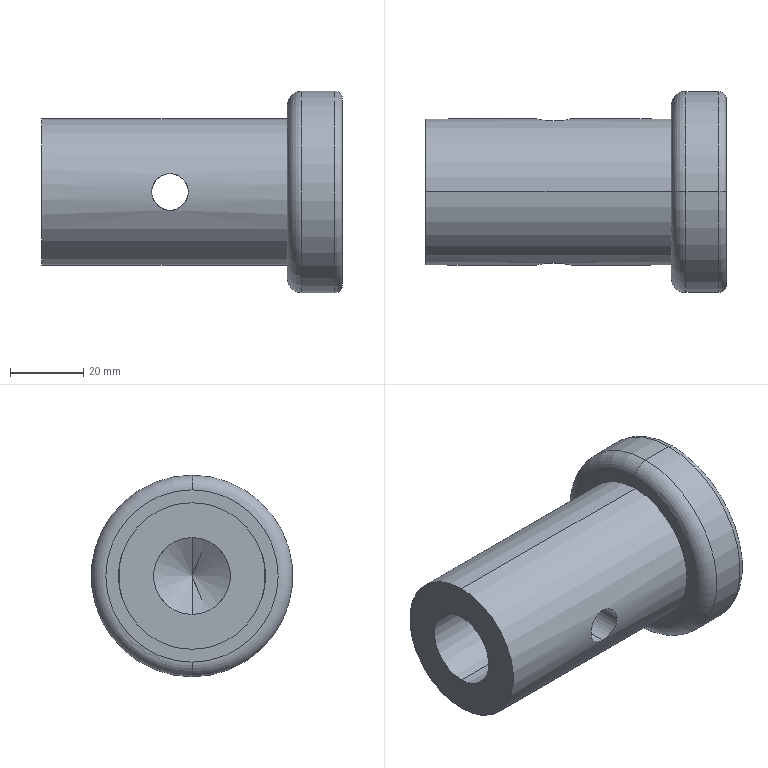Part | SolidWorks | features Fillet 2, HoleWzd 1, ICE 1, Revolution 1 | 1 solid | 21 faces | box 82 x 55 x 55 mm | volume 93090 mm3 | cylinder 10 | torus 4 | plane 3 | cone 2 | sphere 2 | commonest cylinder face diameters 10 x4 21 x2 40 x2 55 x2
STEP:
#1=CARTESIAN_POINT('',(67.,0.,23.5));
#2=VERTEX_POINT('',#1);
#3=CARTESIAN_POINT('',(67.,0.,-23.5));
#4=VERTEX_POINT('',#3);
#5=CARTESIAN_POINT('',(67.,0.,0.));
#6=DIRECTION('',(-1.,0.,0.));
#7=DIRECTION('',(0.,0.,-1.));
#8=AXIS2_PLACEMENT_3D('',#5,#6,#7);
#9=CIRCLE('',#8,23.5);
#10=EDGE_CURVE('',#2,#4,#9,.T.);
#11=ORIENTED_EDGE('',*,*,#10,.F.);
#12=CARTESIAN_POINT('',(71.,0.,27.5));
#13=VERTEX_POINT('',#12);
#14=CARTESIAN_POINT('',(71.,0.,23.5));
#15=DIRECTION('',(0.,1.,0.));
#16=DIRECTION('',(0.,0.,1.));
#17=AXIS2_PLACEMENT_3D('',#14,#15,#16);
#18=CIRCLE('',#17,4.);
#19=EDGE_CURVE('',#2,#13,#18,.T.);
#20=ORIENTED_EDGE('',*,*,#19,.T.);
#21=CARTESIAN_POINT('',(71.,0.,-27.5));
#22=VERTEX_POINT('',#21);
#23=CARTESIAN_POINT('',(71.,0.,0.));
#24=DIRECTION('',(1.,0.,0.));
#25=DIRECTION('',(0.,0.,-1.));
#26=AXIS2_PLACEMENT_3D('',#23,#24,#25);
#27=CIRCLE('',#26,27.5);
#28=EDGE_CURVE('',#22,#13,#27,.T.);
#29=ORIENTED_EDGE('',*,*,#28,.F.);
#30=CARTESIAN_POINT('',(71.,0.,-23.5));
#31=DIRECTION('',(0.,-1.,0.));
#32=DIRECTION('',(0.,0.,-1.));
#33=AXIS2_PLACEMENT_3D('',#30,#31,#32);
#34=CIRCLE('',#33,4.);
#35=EDGE_CURVE('',#4,#22,#34,.T.);
#36=ORIENTED_EDGE('',*,*,#35,.F.);
#37=EDGE_LOOP('',(#11,#20,#29,#36));
#38=FACE_OUTER_BOUND('',#37,.T.);
#39=CARTESIAN_POINT('',(71.,0.,0.));
#40=DIRECTION('',(1.,0.,0.));
#41=DIRECTION('',(0.,0.,-1.));
#42=AXIS2_PLACEMENT_3D('',#39,#40,#41);
#43=TOROIDAL_SURFACE('',#42,23.5,4.);
#44=ADVANCED_FACE('',(#38),#43,.T.);
#45=CARTESIAN_POINT('',(82.,0.,-25.5));
#46=VERTEX_POINT('',#45);
#47=CARTESIAN_POINT('',(82.,0.,25.5));
#48=VERTEX_POINT('',#47);
#49=CARTESIAN_POINT('',(82.,0.,0.));
#50=DIRECTION('',(1.,0.,0.));
#51=DIRECTION('',(0.,0.,1.));
#52=AXIS2_PLACEMENT_3D('',#49,#50,#51);
#53=CIRCLE('',#52,25.5);
#54=EDGE_CURVE('',#46,#48,#53,.T.);
#55=ORIENTED_EDGE('',*,*,#54,.F.);
#56=CARTESIAN_POINT('',(80.,0.,-27.5));
#57=VERTEX_POINT('',#56);
#58=CARTESIAN_POINT('',(80.,0.,-25.5));
#59=DIRECTION('',(0.,1.,0.));
#60=DIRECTION('',(0.,0.,1.));
#61=AXIS2_PLACEMENT_3D('',#58,#59,#60);
#62=CIRCLE('',#61,2.);
#63=EDGE_CURVE('',#46,#57,#62,.T.);
#64=ORIENTED_EDGE('',*,*,#63,.T.);
#65=CARTESIAN_POINT('',(80.,0.,27.5));
#66=VERTEX_POINT('',#65);
#67=CARTESIAN_POINT('',(80.,0.,0.));
#68=DIRECTION('',(-1.,0.,0.));
#69=DIRECTION('',(0.,0.,1.));
#70=AXIS2_PLACEMENT_3D('',#67,#68,#69);
#71=CIRCLE('',#70,27.5);
#72=EDGE_CURVE('',#66,#57,#71,.T.);
#73=ORIENTED_EDGE('',*,*,#72,.F.);
#74=CARTESIAN_POINT('',(80.,0.,25.5));
#75=DIRECTION('',(0.,-1.,0.));
#76=DIRECTION('',(0.,0.,-1.));
#77=AXIS2_PLACEMENT_3D('',#74,#75,#76);
#78=CIRCLE('',#77,2.);
#79=EDGE_CURVE('',#48,#66,#78,.T.);
#80=ORIENTED_EDGE('',*,*,#79,.F.);
#81=EDGE_LOOP('',(#55,#64,#73,#80));
#82=FACE_OUTER_BOUND('',#81,.T.);
#83=CARTESIAN_POINT('',(80.,0.,0.));
#84=DIRECTION('',(-1.,0.,0.));
#85=DIRECTION('',(0.,0.,1.));
#86=AXIS2_PLACEMENT_3D('',#83,#84,#85);
#87=TOROIDAL_SURFACE('',#86,25.5,2.);
#88=ADVANCED_FACE('',(#82),#87,.T.);
#89=CARTESIAN_POINT('',(35.,-19.365,-5.));
#90=VERTEX_POINT('',#89);
#91=CARTESIAN_POINT('',(35.,-19.365,5.));
#92=VERTEX_POINT('',#91);
#93=CARTESIAN_POINT('',(35.,-19.365,-5.));
#94=CARTESIAN_POINT('',(34.673,-19.365,-5.));
#95=CARTESIAN_POINT('',(34.347,-19.373,-4.968));
#96=CARTESIAN_POINT('',(33.697,-19.406,-4.839));
#97=CARTESIAN_POINT('',(33.385,-19.43,-4.743));
#98=CARTESIAN_POINT('',(32.782,-19.489,-4.493));
#99=CARTESIAN_POINT('',(32.49,-19.525,-4.337));
#100=CARTESIAN_POINT('',(31.948,-19.602,-3.974));
#101=CARTESIAN_POINT('',(31.697,-19.643,-3.768));
#102=CARTESIAN_POINT('',(31.236,-19.726,-3.307));
#103=CARTESIAN_POINT('',(31.025,-19.768,-3.051));
#104=CARTESIAN_POINT('',(30.664,-19.844,-2.511));
#105=CARTESIAN_POINT('',(30.51,-19.878,-2.224));
#106=CARTESIAN_POINT('',(30.257,-19.937,-1.616));
#107=CARTESIAN_POINT('',(30.161,-19.96,-1.301));
#108=CARTESIAN_POINT('',(30.065,-19.984,-0.8214));
#109=CARTESIAN_POINT('',(30.041,-19.99,-0.6596));
#110=CARTESIAN_POINT('',(30.008,-19.998,-0.3326));
#111=CARTESIAN_POINT('',(30.,-20.,-0.1664));
#112=CARTESIAN_POINT('',(30.,-20.,0.3283));
#113=CARTESIAN_POINT('',(30.032,-19.992,0.6537));
#114=CARTESIAN_POINT('',(30.16,-19.961,1.296));
#115=CARTESIAN_POINT('',(30.257,-19.937,1.615));
#116=CARTESIAN_POINT('',(30.507,-19.879,2.218));
#117=CARTESIAN_POINT('',(30.661,-19.844,2.505));
#118=CARTESIAN_POINT('',(31.025,-19.768,3.051));
#119=CARTESIAN_POINT('',(31.233,-19.727,3.304));
#120=CARTESIAN_POINT('',(31.692,-19.644,3.763));
#121=CARTESIAN_POINT('',(31.946,-19.602,3.972));
#122=CARTESIAN_POINT('',(32.49,-19.525,4.337));
#123=CARTESIAN_POINT('',(32.777,-19.49,4.49));
#124=CARTESIAN_POINT('',(33.379,-19.43,4.741));
#125=CARTESIAN_POINT('',(33.697,-19.406,4.838));
#126=CARTESIAN_POINT('',(34.341,-19.373,4.967));
#127=CARTESIAN_POINT('',(34.668,-19.365,5.));
#128=CARTESIAN_POINT('',(35.,-19.365,5.));
#129=B_SPLINE_CURVE_WITH_KNOTS('',3,(#93,#94,#95,#96,#97,#98,#99,#100,#101,#102,#103,#104,#105,#106,#107,#108,#109,#110,#111,#112,#113,#114,#115,#116,#117,#118,#119,#120,#121,#122,#123,#124,#125,#126,#127,#128),.UNSPECIFIED.,.F.,.F.,(4,2,2,2,2,2,2,2,2,2,2,2,2,2,2,2,2,4),(0.01569,0.01668,0.01766,0.01864,0.01962,0.0206,0.02158,0.02256,0.02305,0.02354,0.02452,0.0255,0.02648,0.02746,0.02844,0.02942,0.0304,0.03138),.UNSPECIFIED.);
#130=EDGE_CURVE('',#90,#92,#129,.T.);
#131=ORIENTED_EDGE('',*,*,#130,.F.);
#132=CARTESIAN_POINT('',(35.,-9.233,-5.));
#133=VERTEX_POINT('',#132);
#134=CARTESIAN_POINT('',(35.,-25.,-5.));
#135=DIRECTION('',(0.,1.,0.));
#136=VECTOR('',#135,1000.);
#137=LINE('',#134,#136);
#138=EDGE_CURVE('',#90,#133,#137,.T.);
#139=ORIENTED_EDGE('',*,*,#138,.T.);
#140=CARTESIAN_POINT('',(35.,-9.233,5.));
#141=VERTEX_POINT('',#140);
#142=CARTESIAN_POINT('',(35.,-9.233,5.));
#143=CARTESIAN_POINT('',(34.664,-9.233,5.));
#144=CARTESIAN_POINT('',(34.335,-9.251,4.966));
#145=CARTESIAN_POINT('',(33.689,-9.32,4.836));
#146=CARTESIAN_POINT('',(33.37,-9.371,4.738));
#147=CARTESIAN_POINT('',(32.767,-9.495,4.486));
#148=CARTESIAN_POINT('',(32.482,-9.567,4.332));
#149=CARTESIAN_POINT('',(31.943,-9.723,3.97));
#150=CARTESIAN_POINT('',(31.692,-9.805,3.763));
#151=CARTESIAN_POINT('',(31.238,-9.968,3.309));
#152=CARTESIAN_POINT('',(31.031,-10.049,3.059));
#153=CARTESIAN_POINT('',(30.668,-10.197,2.518));
#154=CARTESIAN_POINT('',(30.515,-10.264,2.233));
#155=CARTESIAN_POINT('',(30.326,-10.349,1.783));
#156=CARTESIAN_POINT('',(30.27,-10.374,1.629));
#157=CARTESIAN_POINT('',(30.172,-10.419,1.312));
#158=CARTESIAN_POINT('',(30.131,-10.438,1.15));
#159=CARTESIAN_POINT('',(30.033,-10.484,0.6637));
#160=CARTESIAN_POINT('',(30.,-10.5,0.3355));
#161=CARTESIAN_POINT('',(30.,-10.5,-0.1631));
#162=CARTESIAN_POINT('',(30.008,-10.496,-0.3315));
#163=CARTESIAN_POINT('',(30.041,-10.48,-0.6635));
#164=CARTESIAN_POINT('',(30.066,-10.469,-0.8273));
#165=CARTESIAN_POINT('',(30.164,-10.423,-1.312));
#166=CARTESIAN_POINT('',(30.262,-10.377,-1.63));
#167=CARTESIAN_POINT('',(30.516,-10.263,-2.237));
#168=CARTESIAN_POINT('',(30.671,-10.196,-2.523));
#169=CARTESIAN_POINT('',(31.033,-10.048,-3.061));
#170=CARTESIAN_POINT('',(31.242,-9.966,-3.314));
#171=CARTESIAN_POINT('',(31.697,-9.804,-3.768));
#172=CARTESIAN_POINT('',(31.945,-9.722,-3.972));
#173=CARTESIAN_POINT('',(32.486,-9.566,-4.334));
#174=CARTESIAN_POINT('',(32.773,-9.493,-4.488));
#175=CARTESIAN_POINT('',(33.372,-9.371,-4.739));
#176=CARTESIAN_POINT('',(33.687,-9.32,-4.836));
#177=CARTESIAN_POINT('',(34.34,-9.251,-4.967));
#178=CARTESIAN_POINT('',(34.669,-9.233,-5.));
#179=CARTESIAN_POINT('',(35.,-9.233,-5.));
#180=B_SPLINE_CURVE_WITH_KNOTS('',3,(#142,#143,#144,#145,#146,#147,#148,#149,#150,#151,#152,#153,#154,#155,#156,#157,#158,#159,#160,#161,#162,#163,#164,#165,#166,#167,#168,#169,#170,#171,#172,#173,#174,#175,#176,#177,#178,#179),.UNSPECIFIED.,.F.,.F.,(4,2,2,2,2,2,2,2,2,2,2,2,2,2,2,2,2,2,4),(0.,0.0009922,0.001984,0.002977,0.003969,0.004961,0.005953,0.006449,0.006945,0.007938,0.008434,0.00893,0.009922,0.01091,0.01191,0.0129,0.01389,0.01488,0.01588),.UNSPECIFIED.);
#181=EDGE_CURVE('',#141,#133,#180,.T.);
#182=ORIENTED_EDGE('',*,*,#181,.F.);
#183=CARTESIAN_POINT('',(35.,-25.,5.));
#184=DIRECTION('',(0.,1.,0.));
#185=VECTOR('',#184,1000.);
#186=LINE('',#183,#185);
#187=EDGE_CURVE('',#92,#141,#186,.T.);
#188=ORIENTED_EDGE('',*,*,#187,.F.);
#189=EDGE_LOOP('',(#131,#139,#182,#188));
#190=FACE_OUTER_BOUND('',#189,.T.);
#191=CARTESIAN_POINT('',(35.,-25.,0.));
#192=DIRECTION('',(0.,1.,0.));
#193=DIRECTION('',(0.,0.,1.));
#194=AXIS2_PLACEMENT_3D('',#191,#192,#193);
#195=CYLINDRICAL_SURFACE('',#194,5.);
#196=ADVANCED_FACE('',(#190),#195,.F.);
#197=CARTESIAN_POINT('',(35.,9.233,-5.));
#198=VERTEX_POINT('',#197);
#199=CARTESIAN_POINT('',(35.,9.233,5.));
#200=VERTEX_POINT('',#199);
#201=CARTESIAN_POINT('',(35.,9.233,-5.));
#202=CARTESIAN_POINT('',(34.67,9.233,-5.));
#203=CARTESIAN_POINT('',(34.333,9.252,-4.966));
#204=CARTESIAN_POINT('',(33.686,9.321,-4.835));
#205=CARTESIAN_POINT('',(33.373,9.371,-4.739));
#206=CARTESIAN_POINT('',(32.766,9.495,-4.485));
#207=CARTESIAN_POINT('',(32.48,9.568,-4.33));
#208=CARTESIAN_POINT('',(31.944,9.722,-3.971));
#209=CARTESIAN_POINT('',(31.692,9.806,-3.763));
#210=CARTESIAN_POINT('',(31.236,9.968,-3.307));
#211=CARTESIAN_POINT('',(31.032,10.048,-3.06));
#212=CARTESIAN_POINT('',(30.671,10.196,-2.523));
#213=CARTESIAN_POINT('',(30.514,10.265,-2.232));
#214=CARTESIAN_POINT('',(30.262,10.377,-1.631));
#215=CARTESIAN_POINT('',(30.166,10.422,-1.318));
#216=CARTESIAN_POINT('',(30.067,10.468,-0.8302));
#217=CARTESIAN_POINT('',(30.042,10.48,-0.664));
#218=CARTESIAN_POINT('',(30.008,10.496,-0.3336));
#219=CARTESIAN_POINT('',(29.992,10.504,-0.003189));
#220=CARTESIAN_POINT('',(30.008,10.496,0.3273));
#221=CARTESIAN_POINT('',(30.041,10.481,0.6578));
#222=CARTESIAN_POINT('',(30.066,10.469,0.824));
#223=CARTESIAN_POINT('',(30.164,10.423,1.313));
#224=CARTESIAN_POINT('',(30.261,10.378,1.626));
#225=CARTESIAN_POINT('',(30.513,10.265,2.231));
#226=CARTESIAN_POINT('',(30.671,10.196,2.522));
#227=CARTESIAN_POINT('',(31.031,10.049,3.058));
#228=CARTESIAN_POINT('',(31.237,9.968,3.308));
#229=CARTESIAN_POINT('',(31.696,9.804,3.767));
#230=CARTESIAN_POINT('',(31.944,9.722,3.971));
#231=CARTESIAN_POINT('',(32.345,9.606,4.24));
#232=CARTESIAN_POINT('',(32.483,9.569,4.324));
#233=CARTESIAN_POINT('',(32.77,9.498,4.478));
#234=CARTESIAN_POINT('',(32.919,9.464,4.549));
#235=CARTESIAN_POINT('',(33.371,9.371,4.738));
#236=CARTESIAN_POINT('',(33.682,9.321,4.834));
#237=CARTESIAN_POINT('',(34.328,9.252,4.966));
#238=CARTESIAN_POINT('',(34.665,9.233,5.));
#239=CARTESIAN_POINT('',(35.,9.233,5.));
#240=B_SPLINE_CURVE_WITH_KNOTS('',3,(#201,#202,#203,#204,#205,#206,#207,#208,#209,#210,#211,#212,#213,#214,#215,#216,#217,#218,#219,#220,#221,#222,#223,#224,#225,#226,#227,#228,#229,#230,#231,#232,#233,#234,#235,#236,#237,#238,#239),.UNSPECIFIED.,.F.,.F.,(4,2,2,2,2,2,2,2,2,1,2,2,2,2,2,2,2,2,2,4),(0.01588,0.01687,0.01786,0.01885,0.01984,0.02083,0.02182,0.02281,0.02331,0.0238,0.0243,0.02479,0.02578,0.02677,0.02776,0.02876,0.02925,0.02975,0.03074,0.03173),.UNSPECIFIED.);
#241=EDGE_CURVE('',#198,#200,#240,.T.);
#242=ORIENTED_EDGE('',*,*,#241,.F.);
#243=CARTESIAN_POINT('',(35.,19.365,-5.));
#244=VERTEX_POINT('',#243);
#245=CARTESIAN_POINT('',(35.,-25.,-5.));
#246=DIRECTION('',(0.,1.,0.));
#247=VECTOR('',#246,1000.);
#248=LINE('',#245,#247);
#249=EDGE_CURVE('',#198,#244,#248,.T.);
#250=ORIENTED_EDGE('',*,*,#249,.T.);
#251=CARTESIAN_POINT('',(35.,19.365,5.));
#252=VERTEX_POINT('',#251);
#253=CARTESIAN_POINT('',(35.,19.365,5.));
#254=CARTESIAN_POINT('',(34.668,19.365,5.));
#255=CARTESIAN_POINT('',(34.342,19.373,4.967));
#256=CARTESIAN_POINT('',(33.701,19.406,4.839));
#257=CARTESIAN_POINT('',(33.383,19.43,4.743));
#258=CARTESIAN_POINT('',(32.778,19.49,4.491));
#259=CARTESIAN_POINT('',(32.492,19.525,4.338));
#260=CARTESIAN_POINT('',(31.949,19.602,3.975));
#261=CARTESIAN_POINT('',(31.693,19.644,3.764));
#262=CARTESIAN_POINT('',(31.234,19.726,3.305));
#263=CARTESIAN_POINT('',(31.028,19.767,3.054));
#264=CARTESIAN_POINT('',(30.662,19.844,2.508));
#265=CARTESIAN_POINT('',(30.508,19.879,2.219));
#266=CARTESIAN_POINT('',(30.32,19.922,1.768));
#267=CARTESIAN_POINT('',(30.265,19.935,1.614));
#268=CARTESIAN_POINT('',(30.169,19.958,1.301));
#269=CARTESIAN_POINT('',(30.129,19.968,1.14));
#270=CARTESIAN_POINT('',(30.032,19.992,0.655));
#271=CARTESIAN_POINT('',(30.,20.,0.3296));
#272=CARTESIAN_POINT('',(30.,20.,-0.3256));
#273=CARTESIAN_POINT('',(30.033,19.992,-0.6584));
#274=CARTESIAN_POINT('',(30.161,19.96,-1.301));
#275=CARTESIAN_POINT('',(30.256,19.937,-1.613));
#276=CARTESIAN_POINT('',(30.508,19.879,-2.22));
#277=CARTESIAN_POINT('',(30.664,19.844,-2.511));
#278=CARTESIAN_POINT('',(31.025,19.768,-3.051));
#279=CARTESIAN_POINT('',(31.234,19.726,-3.305));
#280=CARTESIAN_POINT('',(31.697,19.643,-3.768));
#281=CARTESIAN_POINT('',(31.948,19.602,-3.974));
#282=CARTESIAN_POINT('',(32.489,19.525,-4.336));
#283=CARTESIAN_POINT('',(32.782,19.489,-4.493));
#284=CARTESIAN_POINT('',(33.385,19.43,-4.743));
#285=CARTESIAN_POINT('',(33.697,19.406,-4.838));
#286=CARTESIAN_POINT('',(34.18,19.382,-4.935));
#287=CARTESIAN_POINT('',(34.344,19.375,-4.96));
#288=CARTESIAN_POINT('',(34.673,19.367,-4.992));
#289=CARTESIAN_POINT('',(34.836,19.365,-5.));
#290=CARTESIAN_POINT('',(35.,19.365,-5.));
#291=B_SPLINE_CURVE_WITH_KNOTS('',3,(#253,#254,#255,#256,#257,#258,#259,#260,#261,#262,#263,#264,#265,#266,#267,#268,#269,#270,#271,#272,#273,#274,#275,#276,#277,#278,#279,#280,#281,#282,#283,#284,#285,#286,#287,#288,#289,#290),.UNSPECIFIED.,.F.,.F.,(4,2,2,2,2,2,2,2,2,2,2,2,2,2,2,2,2,2,4),(0.,0.0009809,0.001962,0.002943,0.003924,0.004905,0.005885,0.006376,0.006866,0.007847,0.008828,0.009809,0.01079,0.01177,0.01275,0.01373,0.01471,0.0152,0.01569),.UNSPECIFIED.);
#292=EDGE_CURVE('',#252,#244,#291,.T.);
#293=ORIENTED_EDGE('',*,*,#292,.F.);
#294=CARTESIAN_POINT('',(35.,-25.,5.));
#295=DIRECTION('',(0.,1.,0.));
#296=VECTOR('',#295,1000.);
#297=LINE('',#294,#296);
#298=EDGE_CURVE('',#200,#252,#297,.T.);
#299=ORIENTED_EDGE('',*,*,#298,.F.);
#300=EDGE_LOOP('',(#242,#250,#293,#299));
#301=FACE_OUTER_BOUND('',#300,.T.);
#302=CARTESIAN_POINT('',(35.,-25.,0.));
#303=DIRECTION('',(0.,1.,0.));
#304=DIRECTION('',(0.,0.,1.));
#305=AXIS2_PLACEMENT_3D('',#302,#303,#304);
#306=CYLINDRICAL_SURFACE('',#305,5.);
#307=ADVANCED_FACE('',(#301),#306,.F.);
#308=ORIENTED_EDGE('',*,*,#181,.T.);
#309=CARTESIAN_POINT('',(35.,-9.233,-5.));
#310=CARTESIAN_POINT('',(35.33,-9.233,-5.));
#311=CARTESIAN_POINT('',(35.667,-9.252,-4.966));
#312=CARTESIAN_POINT('',(36.314,-9.321,-4.835));
#313=CARTESIAN_POINT('',(36.627,-9.371,-4.739));
#314=CARTESIAN_POINT('',(37.234,-9.495,-4.485));
#315=CARTESIAN_POINT('',(37.52,-9.568,-4.33));
#316=CARTESIAN_POINT('',(38.056,-9.722,-3.971));
#317=CARTESIAN_POINT('',(38.308,-9.806,-3.763));
#318=CARTESIAN_POINT('',(38.764,-9.968,-3.307));
#319=CARTESIAN_POINT('',(38.968,-10.048,-3.06));
#320=CARTESIAN_POINT('',(39.329,-10.196,-2.523));
#321=CARTESIAN_POINT('',(39.486,-10.265,-2.232));
#322=CARTESIAN_POINT('',(39.738,-10.377,-1.631));
#323=CARTESIAN_POINT('',(39.834,-10.422,-1.318));
#324=CARTESIAN_POINT('',(39.933,-10.468,-0.8302));
#325=CARTESIAN_POINT('',(39.958,-10.48,-0.664));
#326=CARTESIAN_POINT('',(39.992,-10.496,-0.3336));
#327=CARTESIAN_POINT('',(40.008,-10.504,-0.003189));
#328=CARTESIAN_POINT('',(39.992,-10.496,0.3273));
#329=CARTESIAN_POINT('',(39.959,-10.481,0.6578));
#330=CARTESIAN_POINT('',(39.934,-10.469,0.824));
#331=CARTESIAN_POINT('',(39.836,-10.423,1.313));
#332=CARTESIAN_POINT('',(39.739,-10.378,1.626));
#333=CARTESIAN_POINT('',(39.487,-10.265,2.231));
#334=CARTESIAN_POINT('',(39.329,-10.196,2.522));
#335=CARTESIAN_POINT('',(38.969,-10.049,3.058));
#336=CARTESIAN_POINT('',(38.763,-9.968,3.308));
#337=CARTESIAN_POINT('',(38.304,-9.804,3.767));
#338=CARTESIAN_POINT('',(38.056,-9.722,3.971));
#339=CARTESIAN_POINT('',(37.655,-9.606,4.24));
#340=CARTESIAN_POINT('',(37.517,-9.569,4.324));
#341=CARTESIAN_POINT('',(37.23,-9.498,4.478));
#342=CARTESIAN_POINT('',(37.081,-9.464,4.549));
#343=CARTESIAN_POINT('',(36.629,-9.371,4.738));
#344=CARTESIAN_POINT('',(36.318,-9.321,4.834));
#345=CARTESIAN_POINT('',(35.672,-9.252,4.966));
#346=CARTESIAN_POINT('',(35.335,-9.233,5.));
#347=CARTESIAN_POINT('',(35.,-9.233,5.));
#348=B_SPLINE_CURVE_WITH_KNOTS('',3,(#309,#310,#311,#312,#313,#314,#315,#316,#317,#318,#319,#320,#321,#322,#323,#324,#325,#326,#327,#328,#329,#330,#331,#332,#333,#334,#335,#336,#337,#338,#339,#340,#341,#342,#343,#344,#345,#346,#347),.UNSPECIFIED.,.F.,.F.,(4,2,2,2,2,2,2,2,2,1,2,2,2,2,2,2,2,2,2,4),(0.01588,0.01687,0.01786,0.01885,0.01984,0.02083,0.02182,0.02281,0.02331,0.0238,0.0243,0.02479,0.02578,0.02677,0.02776,0.02876,0.02925,0.02975,0.03074,0.03173),.UNSPECIFIED.);
#349=EDGE_CURVE('',#133,#141,#348,.T.);
#350=ORIENTED_EDGE('',*,*,#349,.T.);
#351=EDGE_LOOP('',(#308,#350));
#352=FACE_BOUND('',#351,.T.);
#353=CARTESIAN_POINT('',(57.,0.,-10.5));
#354=VERTEX_POINT('',#353);
#355=CARTESIAN_POINT('',(57.,0.,10.5));
#356=VERTEX_POINT('',#355);
#357=CARTESIAN_POINT('',(57.,0.,0.));
#358=DIRECTION('',(-1.,0.,0.));
#359=DIRECTION('',(0.,0.,1.));
#360=AXIS2_PLACEMENT_3D('',#357,#358,#359);
#361=CIRCLE('',#360,10.5);
#362=EDGE_CURVE('',#354,#356,#361,.T.);
#363=ORIENTED_EDGE('',*,*,#362,.F.);
#364=CARTESIAN_POINT('',(0.,0.,-10.5));
#365=VERTEX_POINT('',#364);
#366=CARTESIAN_POINT('',(0.,0.,-10.5));
#367=DIRECTION('',(-1.,0.,0.));
#368=VECTOR('',#367,1000.);
#369=LINE('',#366,#368);
#370=EDGE_CURVE('',#354,#365,#369,.T.);
#371=ORIENTED_EDGE('',*,*,#370,.T.);
#372=CARTESIAN_POINT('',(0.,0.,10.5));
#373=VERTEX_POINT('',#372);
#374=CARTESIAN_POINT('',(0.,0.,0.));
#375=DIRECTION('',(-1.,0.,0.));
#376=DIRECTION('',(0.,0.,1.));
#377=AXIS2_PLACEMENT_3D('',#374,#375,#376);
#378=CIRCLE('',#377,10.5);
#379=EDGE_CURVE('',#365,#373,#378,.T.);
#380=ORIENTED_EDGE('',*,*,#379,.T.);
#381=CARTESIAN_POINT('',(0.,0.,10.5));
#382=DIRECTION('',(-1.,0.,0.));
#383=VECTOR('',#382,1000.);
#384=LINE('',#381,#383);
#385=EDGE_CURVE('',#356,#373,#384,.T.);
#386=ORIENTED_EDGE('',*,*,#385,.F.);
#387=EDGE_LOOP('',(#363,#371,#380,#386));
#388=FACE_OUTER_BOUND('',#387,.T.);
#389=CARTESIAN_POINT('',(0.,0.,0.));
#390=DIRECTION('',(-1.,0.,0.));
#391=DIRECTION('',(0.,0.,1.));
#392=AXIS2_PLACEMENT_3D('',#389,#390,#391);
#393=CYLINDRICAL_SURFACE('',#392,10.5);
#394=ADVANCED_FACE('',(#352,#388),#393,.F.);
#395=CARTESIAN_POINT('',(63.309,0.,0.));
#396=VERTEX_POINT('',#395);
#397=CARTESIAN_POINT('',(57.,0.,10.5));
#398=DIRECTION('',(-0.515,0.,0.8572));
#399=VECTOR('',#398,1000.);
#400=LINE('',#397,#399);
#401=EDGE_CURVE('',#396,#356,#400,.T.);
#402=ORIENTED_EDGE('',*,*,#401,.F.);
#403=CARTESIAN_POINT('',(57.,0.,-10.5));
#404=DIRECTION('',(-0.515,0.,-0.8572));
#405=VECTOR('',#404,1000.);
#406=LINE('',#403,#405);
#407=EDGE_CURVE('',#396,#354,#406,.T.);
#408=ORIENTED_EDGE('',*,*,#407,.T.);
#409=ORIENTED_EDGE('',*,*,#362,.T.);
#410=EDGE_LOOP('',(#402,#408,#409));
#411=FACE_OUTER_BOUND('',#410,.T.);
#412=CARTESIAN_POINT('',(57.,0.,0.));
#413=DIRECTION('',(-1.,0.,0.));
#414=DIRECTION('',(0.,0.,1.));
#415=AXIS2_PLACEMENT_3D('',#412,#413,#414);
#416=CONICAL_SURFACE('',#415,10.5,1.03);
#417=ADVANCED_FACE('',(#411),#416,.F.);
#418=ORIENTED_EDGE('',*,*,#292,.T.);
#419=CARTESIAN_POINT('',(35.,19.365,-5.));
#420=CARTESIAN_POINT('',(35.327,19.365,-5.));
#421=CARTESIAN_POINT('',(35.653,19.373,-4.968));
#422=CARTESIAN_POINT('',(36.303,19.406,-4.839));
#423=CARTESIAN_POINT('',(36.615,19.43,-4.743));
#424=CARTESIAN_POINT('',(37.218,19.489,-4.493));
#425=CARTESIAN_POINT('',(37.51,19.525,-4.337));
#426=CARTESIAN_POINT('',(38.052,19.602,-3.974));
#427=CARTESIAN_POINT('',(38.303,19.643,-3.768));
#428=CARTESIAN_POINT('',(38.764,19.726,-3.307));
#429=CARTESIAN_POINT('',(38.975,19.768,-3.051));
#430=CARTESIAN_POINT('',(39.336,19.844,-2.511));
#431=CARTESIAN_POINT('',(39.49,19.878,-2.224));
#432=CARTESIAN_POINT('',(39.743,19.937,-1.616));
#433=CARTESIAN_POINT('',(39.839,19.96,-1.301));
#434=CARTESIAN_POINT('',(39.935,19.984,-0.8214));
#435=CARTESIAN_POINT('',(39.959,19.99,-0.6596));
#436=CARTESIAN_POINT('',(39.992,19.998,-0.3326));
#437=CARTESIAN_POINT('',(40.,20.,-0.1664));
#438=CARTESIAN_POINT('',(40.,20.,0.3283));
#439=CARTESIAN_POINT('',(39.968,19.992,0.6537));
#440=CARTESIAN_POINT('',(39.84,19.961,1.296));
#441=CARTESIAN_POINT('',(39.743,19.937,1.615));
#442=CARTESIAN_POINT('',(39.493,19.879,2.218));
#443=CARTESIAN_POINT('',(39.339,19.844,2.505));
#444=CARTESIAN_POINT('',(38.975,19.768,3.051));
#445=CARTESIAN_POINT('',(38.767,19.727,3.304));
#446=CARTESIAN_POINT('',(38.308,19.644,3.763));
#447=CARTESIAN_POINT('',(38.054,19.602,3.972));
#448=CARTESIAN_POINT('',(37.51,19.525,4.337));
#449=CARTESIAN_POINT('',(37.223,19.49,4.49));
#450=CARTESIAN_POINT('',(36.621,19.43,4.741));
#451=CARTESIAN_POINT('',(36.303,19.406,4.838));
#452=CARTESIAN_POINT('',(35.659,19.373,4.967));
#453=CARTESIAN_POINT('',(35.332,19.365,5.));
#454=CARTESIAN_POINT('',(35.,19.365,5.));
#455=B_SPLINE_CURVE_WITH_KNOTS('',3,(#419,#420,#421,#422,#423,#424,#425,#426,#427,#428,#429,#430,#431,#432,#433,#434,#435,#436,#437,#438,#439,#440,#441,#442,#443,#444,#445,#446,#447,#448,#449,#450,#451,#452,#453,#454),.UNSPECIFIED.,.F.,.F.,(4,2,2,2,2,2,2,2,2,2,2,2,2,2,2,2,2,4),(0.01569,0.01668,0.01766,0.01864,0.01962,0.0206,0.02158,0.02256,0.02305,0.02354,0.02452,0.0255,0.02648,0.02746,0.02844,0.02942,0.0304,0.03138),.UNSPECIFIED.);
#456=EDGE_CURVE('',#244,#252,#455,.T.);
#457=ORIENTED_EDGE('',*,*,#456,.T.);
#458=EDGE_LOOP('',(#418,#457));
#459=FACE_BOUND('',#458,.T.);
#460=CARTESIAN_POINT('',(67.,0.,20.));
#461=VERTEX_POINT('',#460);
#462=CARTESIAN_POINT('',(67.,0.,-20.));
#463=VERTEX_POINT('',#462);
#464=CARTESIAN_POINT('',(67.,0.,0.));
#465=DIRECTION('',(-1.,0.,0.));
#466=DIRECTION('',(0.,0.,1.));
#467=AXIS2_PLACEMENT_3D('',#464,#465,#466);
#468=CIRCLE('',#467,20.);
#469=EDGE_CURVE('',#461,#463,#468,.T.);
#470=ORIENTED_EDGE('',*,*,#469,.T.);
#471=CARTESIAN_POINT('',(0.,0.,-20.));
#472=VERTEX_POINT('',#471);
#473=CARTESIAN_POINT('',(0.,0.,-20.));
#474=DIRECTION('',(-1.,0.,0.));
#475=VECTOR('',#474,1000.);
#476=LINE('',#473,#475);
#477=EDGE_CURVE('',#463,#472,#476,.T.);
#478=ORIENTED_EDGE('',*,*,#477,.T.);
#479=CARTESIAN_POINT('',(0.,0.,20.));
#480=VERTEX_POINT('',#479);
#481=CARTESIAN_POINT('',(0.,0.,0.));
#482=DIRECTION('',(-1.,0.,0.));
#483=DIRECTION('',(0.,0.,1.));
#484=AXIS2_PLACEMENT_3D('',#481,#482,#483);
#485=CIRCLE('',#484,20.);
#486=EDGE_CURVE('',#480,#472,#485,.T.);
#487=ORIENTED_EDGE('',*,*,#486,.F.);
#488=CARTESIAN_POINT('',(0.,0.,20.));
#489=DIRECTION('',(-1.,0.,0.));
#490=VECTOR('',#489,1000.);
#491=LINE('',#488,#490);
#492=EDGE_CURVE('',#461,#480,#491,.T.);
#493=ORIENTED_EDGE('',*,*,#492,.F.);
#494=EDGE_LOOP('',(#470,#478,#487,#493));
#495=FACE_OUTER_BOUND('',#494,.T.);
#496=CARTESIAN_POINT('',(0.,0.,0.));
#497=DIRECTION('',(-1.,0.,0.));
#498=DIRECTION('',(0.,0.,1.));
#499=AXIS2_PLACEMENT_3D('',#496,#497,#498);
#500=CYLINDRICAL_SURFACE('',#499,20.);
#501=ADVANCED_FACE('',(#459,#495),#500,.T.);
#502=ORIENTED_EDGE('',*,*,#72,.T.);
#503=CARTESIAN_POINT('',(0.,0.,-27.5));
#504=DIRECTION('',(-1.,0.,0.));
#505=VECTOR('',#504,1000.);
#506=LINE('',#503,#505);
#507=EDGE_CURVE('',#57,#22,#506,.T.);
#508=ORIENTED_EDGE('',*,*,#507,.T.);
#509=ORIENTED_EDGE('',*,*,#28,.T.);
#510=CARTESIAN_POINT('',(0.,0.,27.5));
#511=DIRECTION('',(-1.,0.,0.));
#512=VECTOR('',#511,1000.);
#513=LINE('',#510,#512);
#514=EDGE_CURVE('',#66,#13,#513,.T.);
#515=ORIENTED_EDGE('',*,*,#514,.F.);
#516=EDGE_LOOP('',(#502,#508,#509,#515));
#517=FACE_OUTER_BOUND('',#516,.T.);
#518=CARTESIAN_POINT('',(0.,0.,0.));
#519=DIRECTION('',(-1.,0.,0.));
#520=DIRECTION('',(0.,0.,1.));
#521=AXIS2_PLACEMENT_3D('',#518,#519,#520);
#522=CYLINDRICAL_SURFACE('',#521,27.5);
#523=ADVANCED_FACE('',(#517),#522,.T.);
#524=CARTESIAN_POINT('',(82.,24.,0.));
#525=VERTEX_POINT('',#524);
#526=CARTESIAN_POINT('',(82.,-24.,0.));
#527=VERTEX_POINT('',#526);
#528=CARTESIAN_POINT('',(82.,0.,0.));
#529=DIRECTION('',(-1.,0.,0.));
#530=DIRECTION('',(0.,0.,1.));
#531=AXIS2_PLACEMENT_3D('',#528,#529,#530);
#532=CIRCLE('',#531,24.);
#533=EDGE_CURVE('',#525,#527,#532,.T.);
#534=ORIENTED_EDGE('',*,*,#533,.F.);
#535=CARTESIAN_POINT('',(77.589,0.,0.));
#536=VERTEX_POINT('',#535);
#537=CARTESIAN_POINT('',(145.089,0.,0.));
#538=DIRECTION('',(0.,0.,1.));
#539=DIRECTION('',(0.,-1.,0.));
#540=AXIS2_PLACEMENT_3D('',#537,#538,#539);
#541=CIRCLE('',#540,67.5);
#542=EDGE_CURVE('',#525,#536,#541,.T.);
#543=ORIENTED_EDGE('',*,*,#542,.T.);
#544=CARTESIAN_POINT('',(145.089,0.,0.));
#545=DIRECTION('',(0.,0.,-1.));
#546=DIRECTION('',(-1.,0.,0.));
#547=AXIS2_PLACEMENT_3D('',#544,#545,#546);
#548=CIRCLE('',#547,67.5);
#549=EDGE_CURVE('',#527,#536,#548,.T.);
#550=ORIENTED_EDGE('',*,*,#549,.F.);
#551=EDGE_LOOP('',(#534,#543,#550));
#552=FACE_OUTER_BOUND('',#551,.T.);
#553=CARTESIAN_POINT('',(145.089,0.,0.));
#554=DIRECTION('',(0.,0.,1.));
#555=DIRECTION('',(0.,-1.,0.));
#556=AXIS2_PLACEMENT_3D('',#553,#554,#555);
#557=SPHERICAL_SURFACE('',#556,67.5);
#558=ADVANCED_FACE('',(#552),#557,.F.);
#559=CARTESIAN_POINT('',(0.,0.,0.));
#560=DIRECTION('',(-1.,0.,0.));
#561=DIRECTION('',(0.,0.,1.));
#562=AXIS2_PLACEMENT_3D('',#559,#560,#561);
#563=CIRCLE('',#562,10.5);
#564=EDGE_CURVE('',#373,#365,#563,.T.);
#565=ORIENTED_EDGE('',*,*,#564,.F.);
#566=ORIENTED_EDGE('',*,*,#379,.F.);
#567=EDGE_LOOP('',(#565,#566));
#568=FACE_BOUND('',#567,.T.);
#569=ORIENTED_EDGE('',*,*,#486,.T.);
#570=CARTESIAN_POINT('',(0.,0.,0.));
#571=DIRECTION('',(-1.,0.,0.));
#572=DIRECTION('',(0.,0.,1.));
#573=AXIS2_PLACEMENT_3D('',#570,#571,#572);
#574=CIRCLE('',#573,20.);
#575=EDGE_CURVE('',#472,#480,#574,.T.);
#576=ORIENTED_EDGE('',*,*,#575,.T.);
#577=EDGE_LOOP('',(#569,#576));
#578=FACE_OUTER_BOUND('',#577,.T.);
#579=CARTESIAN_POINT('',(0.,0.,0.));
#580=DIRECTION('',(1.,0.,0.));
#581=DIRECTION('',(0.,0.,-1.));
#582=AXIS2_PLACEMENT_3D('',#579,#580,#581);
#583=PLANE('',#582);
#584=ADVANCED_FACE('',(#568,#578),#583,.F.);
#585=ORIENTED_EDGE('',*,*,#542,.F.);
#586=CARTESIAN_POINT('',(82.,0.,0.));
#587=DIRECTION('',(-1.,0.,0.));
#588=DIRECTION('',(0.,0.,1.));
#589=AXIS2_PLACEMENT_3D('',#586,#587,#588);
#590=CIRCLE('',#589,24.);
#591=EDGE_CURVE('',#527,#525,#590,.T.);
#592=ORIENTED_EDGE('',*,*,#591,.F.);
#593=ORIENTED_EDGE('',*,*,#549,.T.);
#594=EDGE_LOOP('',(#585,#592,#593));
#595=FACE_OUTER_BOUND('',#594,.T.);
#596=CARTESIAN_POINT('',(145.089,0.,0.));
#597=DIRECTION('',(0.,0.,1.));
#598=DIRECTION('',(0.,-1.,0.));
#599=AXIS2_PLACEMENT_3D('',#596,#597,#598);
#600=SPHERICAL_SURFACE('',#599,67.5);
#601=ADVANCED_FACE('',(#595),#600,.F.);
#602=CARTESIAN_POINT('',(82.,0.,0.));
#603=DIRECTION('',(1.,0.,0.));
#604=DIRECTION('',(0.,0.,1.));
#605=AXIS2_PLACEMENT_3D('',#602,#603,#604);
#606=CIRCLE('',#605,25.5);
#607=EDGE_CURVE('',#48,#46,#606,.T.);
#608=ORIENTED_EDGE('',*,*,#607,.T.);
#609=ORIENTED_EDGE('',*,*,#54,.T.);
#610=EDGE_LOOP('',(#608,#609));
#611=FACE_OUTER_BOUND('',#610,.T.);
#612=ORIENTED_EDGE('',*,*,#591,.T.);
#613=ORIENTED_EDGE('',*,*,#533,.T.);
#614=EDGE_LOOP('',(#612,#613));
#615=FACE_BOUND('',#614,.T.);
#616=CARTESIAN_POINT('',(82.,24.,0.));
#617=DIRECTION('',(-1.,0.,0.));
#618=DIRECTION('',(0.,0.,1.));
#619=AXIS2_PLACEMENT_3D('',#616,#617,#618);
#620=PLANE('',#619);
#621=ADVANCED_FACE('',(#611,#615),#620,.F.);
#622=ORIENTED_EDGE('',*,*,#507,.F.);
#623=CARTESIAN_POINT('',(80.,0.,0.));
#624=DIRECTION('',(-1.,0.,0.));
#625=DIRECTION('',(0.,0.,1.));
#626=AXIS2_PLACEMENT_3D('',#623,#624,#625);
#627=CIRCLE('',#626,27.5);
#628=EDGE_CURVE('',#57,#66,#627,.T.);
#629=ORIENTED_EDGE('',*,*,#628,.T.);
#630=ORIENTED_EDGE('',*,*,#514,.T.);
#631=CARTESIAN_POINT('',(71.,0.,0.));
#632=DIRECTION('',(1.,0.,0.));
#633=DIRECTION('',(0.,0.,-1.));
#634=AXIS2_PLACEMENT_3D('',#631,#632,#633);
#635=CIRCLE('',#634,27.5);
#636=EDGE_CURVE('',#13,#22,#635,.T.);
#637=ORIENTED_EDGE('',*,*,#636,.T.);
#638=EDGE_LOOP('',(#622,#629,#630,#637));
#639=FACE_OUTER_BOUND('',#638,.T.);
#640=CARTESIAN_POINT('',(0.,0.,0.));
#641=DIRECTION('',(-1.,0.,0.));
#642=DIRECTION('',(0.,0.,1.));
#643=AXIS2_PLACEMENT_3D('',#640,#641,#642);
#644=CYLINDRICAL_SURFACE('',#643,27.5);
#645=ADVANCED_FACE('',(#639),#644,.T.);
#646=CARTESIAN_POINT('',(67.,0.,0.));
#647=DIRECTION('',(-1.,0.,0.));
#648=DIRECTION('',(0.,0.,-1.));
#649=AXIS2_PLACEMENT_3D('',#646,#647,#648);
#650=CIRCLE('',#649,23.5);
#651=EDGE_CURVE('',#4,#2,#650,.T.);
#652=ORIENTED_EDGE('',*,*,#651,.T.);
#653=ORIENTED_EDGE('',*,*,#10,.T.);
#654=EDGE_LOOP('',(#652,#653));
#655=FACE_OUTER_BOUND('',#654,.T.);
#656=ORIENTED_EDGE('',*,*,#469,.F.);
#657=CARTESIAN_POINT('',(67.,0.,0.));
#658=DIRECTION('',(-1.,0.,0.));
#659=DIRECTION('',(0.,0.,1.));
#660=AXIS2_PLACEMENT_3D('',#657,#658,#659);
#661=CIRCLE('',#660,20.);
#662=EDGE_CURVE('',#463,#461,#661,.T.);
#663=ORIENTED_EDGE('',*,*,#662,.F.);
#664=EDGE_LOOP('',(#656,#663));
#665=FACE_BOUND('',#664,.T.);
#666=CARTESIAN_POINT('',(67.,27.5,0.));
#667=DIRECTION('',(1.,0.,0.));
#668=DIRECTION('',(0.,0.,-1.));
#669=AXIS2_PLACEMENT_3D('',#666,#667,#668);
#670=PLANE('',#669);
#671=ADVANCED_FACE('',(#655,#665),#670,.F.);
#672=ORIENTED_EDGE('',*,*,#477,.F.);
#673=ORIENTED_EDGE('',*,*,#662,.T.);
#674=ORIENTED_EDGE('',*,*,#492,.T.);
#675=ORIENTED_EDGE('',*,*,#575,.F.);
#676=EDGE_LOOP('',(#672,#673,#674,#675));
#677=FACE_OUTER_BOUND('',#676,.T.);
#678=CARTESIAN_POINT('',(35.,-19.365,5.));
#679=CARTESIAN_POINT('',(35.332,-19.365,5.));
#680=CARTESIAN_POINT('',(35.658,-19.373,4.967));
#681=CARTESIAN_POINT('',(36.299,-19.406,4.839));
#682=CARTESIAN_POINT('',(36.617,-19.43,4.743));
#683=CARTESIAN_POINT('',(37.222,-19.49,4.491));
#684=CARTESIAN_POINT('',(37.508,-19.525,4.338));
#685=CARTESIAN_POINT('',(38.051,-19.602,3.975));
#686=CARTESIAN_POINT('',(38.307,-19.644,3.764));
#687=CARTESIAN_POINT('',(38.766,-19.726,3.305));
#688=CARTESIAN_POINT('',(38.972,-19.767,3.054));
#689=CARTESIAN_POINT('',(39.338,-19.844,2.508));
#690=CARTESIAN_POINT('',(39.492,-19.879,2.219));
#691=CARTESIAN_POINT('',(39.68,-19.922,1.768));
#692=CARTESIAN_POINT('',(39.735,-19.935,1.614));
#693=CARTESIAN_POINT('',(39.831,-19.958,1.301));
#694=CARTESIAN_POINT('',(39.871,-19.968,1.14));
#695=CARTESIAN_POINT('',(39.968,-19.992,0.655));
#696=CARTESIAN_POINT('',(40.,-20.,0.3296));
#697=CARTESIAN_POINT('',(40.,-20.,-0.3256));
#698=CARTESIAN_POINT('',(39.967,-19.992,-0.6584));
#699=CARTESIAN_POINT('',(39.839,-19.96,-1.301));
#700=CARTESIAN_POINT('',(39.744,-19.937,-1.613));
#701=CARTESIAN_POINT('',(39.492,-19.879,-2.22));
#702=CARTESIAN_POINT('',(39.336,-19.844,-2.511));
#703=CARTESIAN_POINT('',(38.975,-19.768,-3.051));
#704=CARTESIAN_POINT('',(38.766,-19.726,-3.305));
#705=CARTESIAN_POINT('',(38.303,-19.643,-3.768));
#706=CARTESIAN_POINT('',(38.052,-19.602,-3.974));
#707=CARTESIAN_POINT('',(37.511,-19.525,-4.336));
#708=CARTESIAN_POINT('',(37.218,-19.489,-4.493));
#709=CARTESIAN_POINT('',(36.615,-19.43,-4.743));
#710=CARTESIAN_POINT('',(36.303,-19.406,-4.838));
#711=CARTESIAN_POINT('',(35.82,-19.382,-4.935));
#712=CARTESIAN_POINT('',(35.656,-19.375,-4.96));
#713=CARTESIAN_POINT('',(35.327,-19.367,-4.992));
#714=CARTESIAN_POINT('',(35.164,-19.365,-5.));
#715=CARTESIAN_POINT('',(35.,-19.365,-5.));
#716=B_SPLINE_CURVE_WITH_KNOTS('',3,(#678,#679,#680,#681,#682,#683,#684,#685,#686,#687,#688,#689,#690,#691,#692,#693,#694,#695,#696,#697,#698,#699,#700,#701,#702,#703,#704,#705,#706,#707,#708,#709,#710,#711,#712,#713,#714,#715),.UNSPECIFIED.,.F.,.F.,(4,2,2,2,2,2,2,2,2,2,2,2,2,2,2,2,2,2,4),(0.,0.0009809,0.001962,0.002943,0.003924,0.004905,0.005885,0.006376,0.006866,0.007847,0.008828,0.009809,0.01079,0.01177,0.01275,0.01373,0.01471,0.0152,0.01569),.UNSPECIFIED.);
#717=EDGE_CURVE('',#92,#90,#716,.T.);
#718=ORIENTED_EDGE('',*,*,#717,.T.);
#719=ORIENTED_EDGE('',*,*,#130,.T.);
#720=EDGE_LOOP('',(#718,#719));
#721=FACE_BOUND('',#720,.T.);
#722=CARTESIAN_POINT('',(0.,0.,0.));
#723=DIRECTION('',(-1.,0.,0.));
#724=DIRECTION('',(0.,0.,1.));
#725=AXIS2_PLACEMENT_3D('',#722,#723,#724);
#726=CYLINDRICAL_SURFACE('',#725,20.);
#727=ADVANCED_FACE('',(#677,#721),#726,.T.);
#728=ORIENTED_EDGE('',*,*,#407,.F.);
#729=ORIENTED_EDGE('',*,*,#401,.T.);
#730=CARTESIAN_POINT('',(57.,0.,0.));
#731=DIRECTION('',(-1.,0.,0.));
#732=DIRECTION('',(0.,0.,1.));
#733=AXIS2_PLACEMENT_3D('',#730,#731,#732);
#734=CIRCLE('',#733,10.5);
#735=EDGE_CURVE('',#356,#354,#734,.T.);
#736=ORIENTED_EDGE('',*,*,#735,.T.);
#737=EDGE_LOOP('',(#728,#729,#736));
#738=FACE_OUTER_BOUND('',#737,.T.);
#739=CARTESIAN_POINT('',(57.,0.,0.));
#740=DIRECTION('',(-1.,0.,0.));
#741=DIRECTION('',(0.,0.,1.));
#742=AXIS2_PLACEMENT_3D('',#739,#740,#741);
#743=CONICAL_SURFACE('',#742,10.5,1.03);
#744=ADVANCED_FACE('',(#738),#743,.F.);
#745=ORIENTED_EDGE('',*,*,#370,.F.);
#746=ORIENTED_EDGE('',*,*,#735,.F.);
#747=ORIENTED_EDGE('',*,*,#385,.T.);
#748=ORIENTED_EDGE('',*,*,#564,.T.);
#749=EDGE_LOOP('',(#745,#746,#747,#748));
#750=FACE_OUTER_BOUND('',#749,.T.);
#751=CARTESIAN_POINT('',(35.,9.233,5.));
#752=CARTESIAN_POINT('',(35.336,9.233,5.));
#753=CARTESIAN_POINT('',(35.665,9.251,4.966));
#754=CARTESIAN_POINT('',(36.311,9.32,4.836));
#755=CARTESIAN_POINT('',(36.63,9.371,4.738));
#756=CARTESIAN_POINT('',(37.233,9.495,4.486));
#757=CARTESIAN_POINT('',(37.518,9.567,4.332));
#758=CARTESIAN_POINT('',(38.057,9.723,3.97));
#759=CARTESIAN_POINT('',(38.308,9.805,3.763));
#760=CARTESIAN_POINT('',(38.762,9.968,3.309));
#761=CARTESIAN_POINT('',(38.969,10.049,3.059));
#762=CARTESIAN_POINT('',(39.332,10.197,2.518));
#763=CARTESIAN_POINT('',(39.485,10.264,2.233));
#764=CARTESIAN_POINT('',(39.674,10.349,1.783));
#765=CARTESIAN_POINT('',(39.73,10.374,1.629));
#766=CARTESIAN_POINT('',(39.828,10.419,1.312));
#767=CARTESIAN_POINT('',(39.869,10.438,1.15));
#768=CARTESIAN_POINT('',(39.967,10.484,0.6637));
#769=CARTESIAN_POINT('',(40.,10.5,0.3355));
#770=CARTESIAN_POINT('',(40.,10.5,-0.1631));
#771=CARTESIAN_POINT('',(39.992,10.496,-0.3315));
#772=CARTESIAN_POINT('',(39.959,10.48,-0.6635));
#773=CARTESIAN_POINT('',(39.934,10.469,-0.8273));
#774=CARTESIAN_POINT('',(39.836,10.423,-1.312));
#775=CARTESIAN_POINT('',(39.738,10.377,-1.63));
#776=CARTESIAN_POINT('',(39.484,10.263,-2.237));
#777=CARTESIAN_POINT('',(39.329,10.196,-2.523));
#778=CARTESIAN_POINT('',(38.967,10.048,-3.061));
#779=CARTESIAN_POINT('',(38.758,9.966,-3.314));
#780=CARTESIAN_POINT('',(38.303,9.804,-3.768));
#781=CARTESIAN_POINT('',(38.055,9.722,-3.972));
#782=CARTESIAN_POINT('',(37.514,9.566,-4.334));
#783=CARTESIAN_POINT('',(37.227,9.493,-4.488));
#784=CARTESIAN_POINT('',(36.628,9.371,-4.739));
#785=CARTESIAN_POINT('',(36.313,9.32,-4.836));
#786=CARTESIAN_POINT('',(35.66,9.251,-4.967));
#787=CARTESIAN_POINT('',(35.331,9.233,-5.));
#788=CARTESIAN_POINT('',(35.,9.233,-5.));
#789=B_SPLINE_CURVE_WITH_KNOTS('',3,(#751,#752,#753,#754,#755,#756,#757,#758,#759,#760,#761,#762,#763,#764,#765,#766,#767,#768,#769,#770,#771,#772,#773,#774,#775,#776,#777,#778,#779,#780,#781,#782,#783,#784,#785,#786,#787,#788),.UNSPECIFIED.,.F.,.F.,(4,2,2,2,2,2,2,2,2,2,2,2,2,2,2,2,2,2,4),(0.,0.0009922,0.001984,0.002977,0.003969,0.004961,0.005953,0.006449,0.006945,0.007938,0.008434,0.00893,0.009922,0.01091,0.01191,0.0129,0.01389,0.01488,0.01588),.UNSPECIFIED.);
#790=EDGE_CURVE('',#200,#198,#789,.T.);
#791=ORIENTED_EDGE('',*,*,#790,.T.);
#792=ORIENTED_EDGE('',*,*,#241,.T.);
#793=EDGE_LOOP('',(#791,#792));
#794=FACE_BOUND('',#793,.T.);
#795=CARTESIAN_POINT('',(0.,0.,0.));
#796=DIRECTION('',(-1.,0.,0.));
#797=DIRECTION('',(0.,0.,1.));
#798=AXIS2_PLACEMENT_3D('',#795,#796,#797);
#799=CYLINDRICAL_SURFACE('',#798,10.5);
#800=ADVANCED_FACE('',(#750,#794),#799,.F.);
#801=ORIENTED_EDGE('',*,*,#249,.F.);
#802=ORIENTED_EDGE('',*,*,#790,.F.);
#803=ORIENTED_EDGE('',*,*,#298,.T.);
#804=ORIENTED_EDGE('',*,*,#456,.F.);
#805=EDGE_LOOP('',(#801,#802,#803,#804));
#806=FACE_OUTER_BOUND('',#805,.T.);
#807=CARTESIAN_POINT('',(35.,-25.,0.));
#808=DIRECTION('',(0.,1.,0.));
#809=DIRECTION('',(0.,0.,1.));
#810=AXIS2_PLACEMENT_3D('',#807,#808,#809);
#811=CYLINDRICAL_SURFACE('',#810,5.);
#812=ADVANCED_FACE('',(#806),#811,.F.);
#813=ORIENTED_EDGE('',*,*,#138,.F.);
#814=ORIENTED_EDGE('',*,*,#717,.F.);
#815=ORIENTED_EDGE('',*,*,#187,.T.);
#816=ORIENTED_EDGE('',*,*,#349,.F.);
#817=EDGE_LOOP('',(#813,#814,#815,#816));
#818=FACE_OUTER_BOUND('',#817,.T.);
#819=CARTESIAN_POINT('',(35.,-25.,0.));
#820=DIRECTION('',(0.,1.,0.));
#821=DIRECTION('',(0.,0.,1.));
#822=AXIS2_PLACEMENT_3D('',#819,#820,#821);
#823=CYLINDRICAL_SURFACE('',#822,5.);
#824=ADVANCED_FACE('',(#818),#823,.F.);
#825=ORIENTED_EDGE('',*,*,#63,.F.);
#826=ORIENTED_EDGE('',*,*,#607,.F.);
#827=ORIENTED_EDGE('',*,*,#79,.T.);
#828=ORIENTED_EDGE('',*,*,#628,.F.);
#829=EDGE_LOOP('',(#825,#826,#827,#828));
#830=FACE_OUTER_BOUND('',#829,.T.);
#831=CARTESIAN_POINT('',(80.,0.,0.));
#832=DIRECTION('',(-1.,0.,0.));
#833=DIRECTION('',(0.,0.,1.));
#834=AXIS2_PLACEMENT_3D('',#831,#832,#833);
#835=TOROIDAL_SURFACE('',#834,25.5,2.);
#836=ADVANCED_FACE('',(#830),#835,.T.);
#837=ORIENTED_EDGE('',*,*,#19,.F.);
#838=ORIENTED_EDGE('',*,*,#651,.F.);
#839=ORIENTED_EDGE('',*,*,#35,.T.);
#840=ORIENTED_EDGE('',*,*,#636,.F.);
#841=EDGE_LOOP('',(#837,#838,#839,#840));
#842=FACE_OUTER_BOUND('',#841,.T.);
#843=CARTESIAN_POINT('',(71.,0.,0.));
#844=DIRECTION('',(1.,0.,0.));
#845=DIRECTION('',(0.,0.,-1.));
#846=AXIS2_PLACEMENT_3D('',#843,#844,#845);
#847=TOROIDAL_SURFACE('',#846,23.5,4.);
#848=ADVANCED_FACE('',(#842),#847,.T.);
#849=CLOSED_SHELL('',(#44,#88,#196,#307,#394,#417,#501,#523,#558,#584,#601,#621,#645,#671,#727,#744,#800,#812,#824,#836,#848));
#850=MANIFOLD_SOLID_BREP('',#849);
#851=CARTESIAN_POINT('',(0.,0.,0.));
#852=DIRECTION('',(0.,0.,1.));
#853=DIRECTION('',(1.,0.,0.));
#854=AXIS2_PLACEMENT_3D('',#851,#852,#853);
#855=(LENGTH_UNIT()NAMED_UNIT(*)SI_UNIT(.MILLI.,.METRE.));
#856=UNCERTAINTY_MEASURE_WITH_UNIT(LENGTH_MEASURE(0.00001),#855,'','');
#857=(NAMED_UNIT(*)PLANE_ANGLE_UNIT()SI_UNIT($,.RADIAN.));
#858=(NAMED_UNIT(*)SI_UNIT($,.STERADIAN.)SOLID_ANGLE_UNIT());
#859=(GEOMETRIC_REPRESENTATION_CONTEXT(3)GLOBAL_UNCERTAINTY_ASSIGNED_CONTEXT((#856))GLOBAL_UNIT_ASSIGNED_CONTEXT((#855,#857,#858))REPRESENTATION_CONTEXT('',''));
#860=ADVANCED_BREP_SHAPE_REPRESENTATION('',(#850,#854),#859);